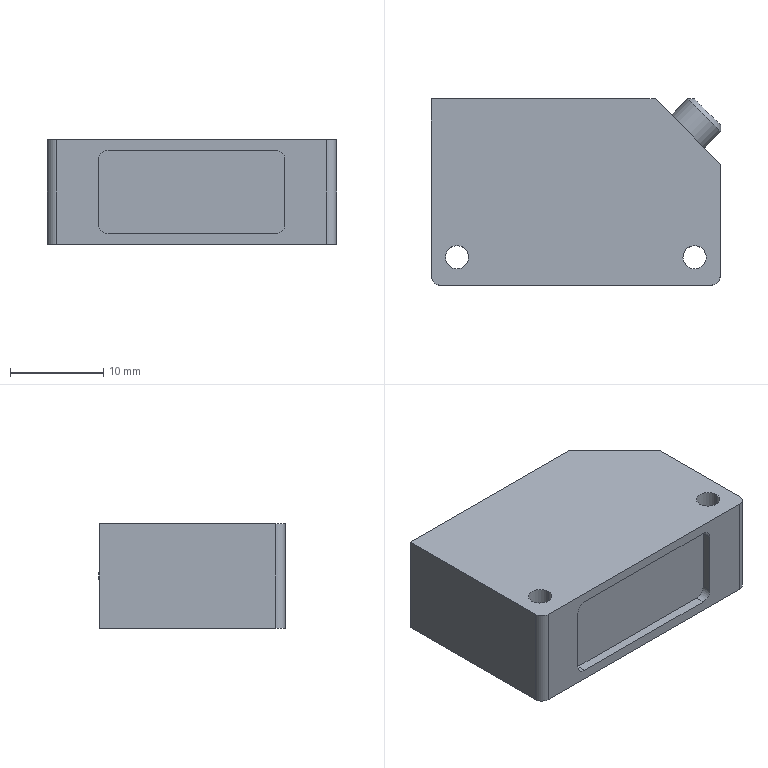Part | STEP file | CX421 | 1 solid | 27 faces | box 31.036 x 20.036 x 11.2 mm | volume 6433 mm3 | plane 13 | cylinder 12 | cone 2 | commonest cylinder face diameters 2 x6 2.5 x4 5 x2